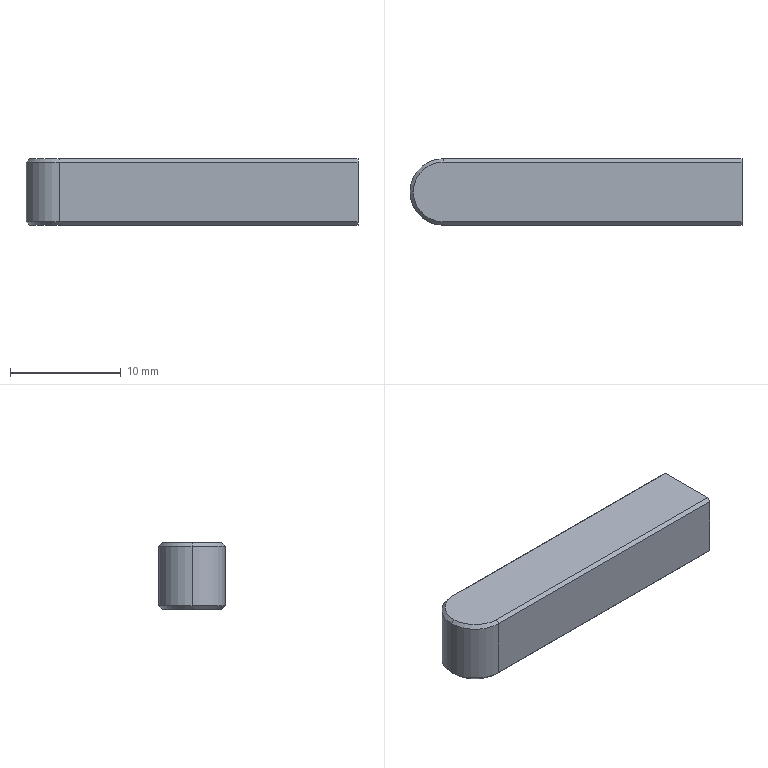Part | SolidWorks | features Chamfer 1, Extrusion 1, Fillet 1 | 1 solid | 15 faces | box 30 x 6 x 6 mm | volume 1051 mm3 | plane 9 | cone 4 | cylinder 2 | commonest cylinder face diameters 6 x2
STEP:
#1=CARTESIAN_POINT('',(15.,-2.7,0.));
#2=VERTEX_POINT('',#1);
#3=CARTESIAN_POINT('',(15.,2.7,0.));
#4=VERTEX_POINT('',#3);
#5=CARTESIAN_POINT('',(15.,3.,0.));
#6=DIRECTION('',(0.,1.,0.));
#7=VECTOR('',#6,1000.);
#8=LINE('',#5,#7);
#9=EDGE_CURVE('',#2,#4,#8,.T.);
#10=ORIENTED_EDGE('',*,*,#9,.T.);
#11=CARTESIAN_POINT('',(15.,3.,0.3));
#12=VERTEX_POINT('',#11);
#13=CARTESIAN_POINT('',(15.,3.,0.3));
#14=DIRECTION('',(0.,0.7071,0.7071));
#15=VECTOR('',#14,1000.);
#16=LINE('',#13,#15);
#17=EDGE_CURVE('',#4,#12,#16,.T.);
#18=ORIENTED_EDGE('',*,*,#17,.T.);
#19=CARTESIAN_POINT('',(15.,3.,5.7));
#20=VERTEX_POINT('',#19);
#21=CARTESIAN_POINT('',(15.,3.,6.));
#22=DIRECTION('',(0.,0.,-1.));
#23=VECTOR('',#22,1000.);
#24=LINE('',#21,#23);
#25=EDGE_CURVE('',#20,#12,#24,.T.);
#26=ORIENTED_EDGE('',*,*,#25,.F.);
#27=CARTESIAN_POINT('',(15.,2.7,6.));
#28=VERTEX_POINT('',#27);
#29=CARTESIAN_POINT('',(15.,2.7,6.));
#30=DIRECTION('',(0.,-0.7071,0.7071));
#31=VECTOR('',#30,1000.);
#32=LINE('',#29,#31);
#33=EDGE_CURVE('',#20,#28,#32,.T.);
#34=ORIENTED_EDGE('',*,*,#33,.T.);
#35=CARTESIAN_POINT('',(15.,-2.7,6.));
#36=VERTEX_POINT('',#35);
#37=CARTESIAN_POINT('',(15.,3.,6.));
#38=DIRECTION('',(0.,1.,0.));
#39=VECTOR('',#38,1000.);
#40=LINE('',#37,#39);
#41=EDGE_CURVE('',#36,#28,#40,.T.);
#42=ORIENTED_EDGE('',*,*,#41,.F.);
#43=CARTESIAN_POINT('',(15.,-3.,5.7));
#44=VERTEX_POINT('',#43);
#45=CARTESIAN_POINT('',(15.,-2.7,6.));
#46=DIRECTION('',(0.,-0.7071,-0.7071));
#47=VECTOR('',#46,1000.);
#48=LINE('',#45,#47);
#49=EDGE_CURVE('',#36,#44,#48,.T.);
#50=ORIENTED_EDGE('',*,*,#49,.T.);
#51=CARTESIAN_POINT('',(15.,-3.,0.3));
#52=VERTEX_POINT('',#51);
#53=CARTESIAN_POINT('',(15.,-3.,6.));
#54=DIRECTION('',(0.,0.,-1.));
#55=VECTOR('',#54,1000.);
#56=LINE('',#53,#55);
#57=EDGE_CURVE('',#44,#52,#56,.T.);
#58=ORIENTED_EDGE('',*,*,#57,.T.);
#59=CARTESIAN_POINT('',(15.,-3.,0.3));
#60=DIRECTION('',(0.,0.7071,-0.7071));
#61=VECTOR('',#60,1000.);
#62=LINE('',#59,#61);
#63=EDGE_CURVE('',#52,#2,#62,.T.);
#64=ORIENTED_EDGE('',*,*,#63,.T.);
#65=EDGE_LOOP('',(#10,#18,#26,#34,#42,#50,#58,#64));
#66=FACE_OUTER_BOUND('',#65,.T.);
#67=CARTESIAN_POINT('',(15.,3.,6.));
#68=DIRECTION('',(-1.,0.,0.));
#69=DIRECTION('',(0.,0.,1.));
#70=AXIS2_PLACEMENT_3D('',#67,#68,#69);
#71=PLANE('',#70);
#72=ADVANCED_FACE('',(#66),#71,.F.);
#73=ORIENTED_EDGE('',*,*,#25,.T.);
#74=CARTESIAN_POINT('',(-12.,3.,0.3));
#75=VERTEX_POINT('',#74);
#76=CARTESIAN_POINT('',(-15.,3.,0.3));
#77=DIRECTION('',(-1.,0.,0.));
#78=VECTOR('',#77,1000.);
#79=LINE('',#76,#78);
#80=EDGE_CURVE('',#12,#75,#79,.T.);
#81=ORIENTED_EDGE('',*,*,#80,.T.);
#82=CARTESIAN_POINT('',(-12.,3.,5.7));
#83=VERTEX_POINT('',#82);
#84=CARTESIAN_POINT('',(-12.,3.,6.));
#85=DIRECTION('',(0.,0.,1.));
#86=VECTOR('',#85,1000.);
#87=LINE('',#84,#86);
#88=EDGE_CURVE('',#75,#83,#87,.T.);
#89=ORIENTED_EDGE('',*,*,#88,.T.);
#90=CARTESIAN_POINT('',(15.,3.,5.7));
#91=DIRECTION('',(1.,0.,0.));
#92=VECTOR('',#91,1000.);
#93=LINE('',#90,#92);
#94=EDGE_CURVE('',#83,#20,#93,.T.);
#95=ORIENTED_EDGE('',*,*,#94,.T.);
#96=EDGE_LOOP('',(#73,#81,#89,#95));
#97=FACE_OUTER_BOUND('',#96,.T.);
#98=CARTESIAN_POINT('',(-15.,3.,6.));
#99=DIRECTION('',(0.,-1.,0.));
#100=DIRECTION('',(0.,0.,-1.));
#101=AXIS2_PLACEMENT_3D('',#98,#99,#100);
#102=PLANE('',#101);
#103=ADVANCED_FACE('',(#97),#102,.F.);
#104=CARTESIAN_POINT('',(-12.,-3.,5.7));
#105=VERTEX_POINT('',#104);
#106=CARTESIAN_POINT('',(-12.,-3.,0.3));
#107=VERTEX_POINT('',#106);
#108=CARTESIAN_POINT('',(-12.,-3.,6.));
#109=DIRECTION('',(0.,0.,-1.));
#110=VECTOR('',#109,1000.);
#111=LINE('',#108,#110);
#112=EDGE_CURVE('',#105,#107,#111,.T.);
#113=ORIENTED_EDGE('',*,*,#112,.T.);
#114=CARTESIAN_POINT('',(-15.,-3.,0.3));
#115=DIRECTION('',(1.,0.,0.));
#116=VECTOR('',#115,1000.);
#117=LINE('',#114,#116);
#118=EDGE_CURVE('',#107,#52,#117,.T.);
#119=ORIENTED_EDGE('',*,*,#118,.T.);
#120=ORIENTED_EDGE('',*,*,#57,.F.);
#121=CARTESIAN_POINT('',(-12.,-3.,5.7));
#122=DIRECTION('',(-1.,0.,0.));
#123=VECTOR('',#122,1000.);
#124=LINE('',#121,#123);
#125=EDGE_CURVE('',#44,#105,#124,.T.);
#126=ORIENTED_EDGE('',*,*,#125,.T.);
#127=EDGE_LOOP('',(#113,#119,#120,#126));
#128=FACE_OUTER_BOUND('',#127,.T.);
#129=CARTESIAN_POINT('',(-15.,-3.,6.));
#130=DIRECTION('',(0.,1.,0.));
#131=DIRECTION('',(0.,0.,1.));
#132=AXIS2_PLACEMENT_3D('',#129,#130,#131);
#133=PLANE('',#132);
#134=ADVANCED_FACE('',(#128),#133,.F.);
#135=ORIENTED_EDGE('',*,*,#41,.T.);
#136=CARTESIAN_POINT('',(-12.,2.7,6.));
#137=VERTEX_POINT('',#136);
#138=CARTESIAN_POINT('',(-12.,2.7,6.));
#139=DIRECTION('',(-1.,0.,0.));
#140=VECTOR('',#139,1000.);
#141=LINE('',#138,#140);
#142=EDGE_CURVE('',#28,#137,#141,.T.);
#143=ORIENTED_EDGE('',*,*,#142,.T.);
#144=CARTESIAN_POINT('',(-14.7,0.,6.));
#145=VERTEX_POINT('',#144);
#146=CARTESIAN_POINT('',(-12.,0.,6.));
#147=DIRECTION('',(0.,0.,1.));
#148=DIRECTION('',(1.,0.,0.));
#149=AXIS2_PLACEMENT_3D('',#146,#147,#148);
#150=CIRCLE('',#149,2.7);
#151=EDGE_CURVE('',#137,#145,#150,.T.);
#152=ORIENTED_EDGE('',*,*,#151,.T.);
#153=CARTESIAN_POINT('',(-12.,-2.7,6.));
#154=VERTEX_POINT('',#153);
#155=CARTESIAN_POINT('',(-12.,0.,6.));
#156=DIRECTION('',(0.,0.,1.));
#157=DIRECTION('',(1.,0.,0.));
#158=AXIS2_PLACEMENT_3D('',#155,#156,#157);
#159=CIRCLE('',#158,2.7);
#160=EDGE_CURVE('',#145,#154,#159,.T.);
#161=ORIENTED_EDGE('',*,*,#160,.T.);
#162=CARTESIAN_POINT('',(15.,-2.7,6.));
#163=DIRECTION('',(1.,0.,0.));
#164=VECTOR('',#163,1000.);
#165=LINE('',#162,#164);
#166=EDGE_CURVE('',#154,#36,#165,.T.);
#167=ORIENTED_EDGE('',*,*,#166,.T.);
#168=EDGE_LOOP('',(#135,#143,#152,#161,#167));
#169=FACE_OUTER_BOUND('',#168,.T.);
#170=CARTESIAN_POINT('',(0.,0.,6.));
#171=DIRECTION('',(0.,0.,1.));
#172=DIRECTION('',(1.,0.,0.));
#173=AXIS2_PLACEMENT_3D('',#170,#171,#172);
#174=PLANE('',#173);
#175=ADVANCED_FACE('',(#169),#174,.T.);
#176=CARTESIAN_POINT('',(-14.7,0.,0.));
#177=VERTEX_POINT('',#176);
#178=CARTESIAN_POINT('',(-12.,2.7,0.));
#179=VERTEX_POINT('',#178);
#180=CARTESIAN_POINT('',(-12.,0.,0.));
#181=DIRECTION('',(0.,0.,-1.));
#182=DIRECTION('',(1.,0.,0.));
#183=AXIS2_PLACEMENT_3D('',#180,#181,#182);
#184=CIRCLE('',#183,2.7);
#185=EDGE_CURVE('',#177,#179,#184,.T.);
#186=ORIENTED_EDGE('',*,*,#185,.T.);
#187=CARTESIAN_POINT('',(0.,2.7,0.));
#188=DIRECTION('',(1.,0.,0.));
#189=VECTOR('',#188,1000.);
#190=LINE('',#187,#189);
#191=EDGE_CURVE('',#179,#4,#190,.T.);
#192=ORIENTED_EDGE('',*,*,#191,.T.);
#193=ORIENTED_EDGE('',*,*,#9,.F.);
#194=CARTESIAN_POINT('',(-12.,-2.7,0.));
#195=VERTEX_POINT('',#194);
#196=CARTESIAN_POINT('',(0.,-2.7,0.));
#197=DIRECTION('',(-1.,0.,0.));
#198=VECTOR('',#197,1000.);
#199=LINE('',#196,#198);
#200=EDGE_CURVE('',#2,#195,#199,.T.);
#201=ORIENTED_EDGE('',*,*,#200,.T.);
#202=CARTESIAN_POINT('',(-12.,0.,0.));
#203=DIRECTION('',(0.,0.,-1.));
#204=DIRECTION('',(1.,0.,0.));
#205=AXIS2_PLACEMENT_3D('',#202,#203,#204);
#206=CIRCLE('',#205,2.7);
#207=EDGE_CURVE('',#195,#177,#206,.T.);
#208=ORIENTED_EDGE('',*,*,#207,.T.);
#209=EDGE_LOOP('',(#186,#192,#193,#201,#208));
#210=FACE_OUTER_BOUND('',#209,.T.);
#211=CARTESIAN_POINT('',(0.,0.,0.));
#212=DIRECTION('',(0.,0.,1.));
#213=DIRECTION('',(1.,0.,0.));
#214=AXIS2_PLACEMENT_3D('',#211,#212,#213);
#215=PLANE('',#214);
#216=ADVANCED_FACE('',(#210),#215,.F.);
#217=CARTESIAN_POINT('',(-15.,0.,0.3));
#218=VERTEX_POINT('',#217);
#219=CARTESIAN_POINT('',(-15.,0.,5.7));
#220=VERTEX_POINT('',#219);
#221=CARTESIAN_POINT('',(-15.,0.,6.));
#222=DIRECTION('',(0.,0.,1.));
#223=VECTOR('',#222,1000.);
#224=LINE('',#221,#223);
#225=EDGE_CURVE('',#218,#220,#224,.T.);
#226=ORIENTED_EDGE('',*,*,#225,.F.);
#227=CARTESIAN_POINT('',(-12.,0.,0.3));
#228=DIRECTION('',(0.,0.,1.));
#229=DIRECTION('',(1.,0.,0.));
#230=AXIS2_PLACEMENT_3D('',#227,#228,#229);
#231=CIRCLE('',#230,3.);
#232=EDGE_CURVE('',#218,#107,#231,.T.);
#233=ORIENTED_EDGE('',*,*,#232,.T.);
#234=ORIENTED_EDGE('',*,*,#112,.F.);
#235=CARTESIAN_POINT('',(-12.,0.,5.7));
#236=DIRECTION('',(0.,0.,-1.));
#237=DIRECTION('',(1.,0.,0.));
#238=AXIS2_PLACEMENT_3D('',#235,#236,#237);
#239=CIRCLE('',#238,3.);
#240=EDGE_CURVE('',#105,#220,#239,.T.);
#241=ORIENTED_EDGE('',*,*,#240,.T.);
#242=EDGE_LOOP('',(#226,#233,#234,#241));
#243=FACE_OUTER_BOUND('',#242,.T.);
#244=CARTESIAN_POINT('',(-12.,0.,6.));
#245=DIRECTION('',(0.,0.,-1.));
#246=DIRECTION('',(-1.,0.,0.));
#247=AXIS2_PLACEMENT_3D('',#244,#245,#246);
#248=CYLINDRICAL_SURFACE('',#247,3.);
#249=ADVANCED_FACE('',(#243),#248,.T.);
#250=ORIENTED_EDGE('',*,*,#88,.F.);
#251=CARTESIAN_POINT('',(-12.,0.,0.3));
#252=DIRECTION('',(0.,0.,1.));
#253=DIRECTION('',(1.,0.,0.));
#254=AXIS2_PLACEMENT_3D('',#251,#252,#253);
#255=CIRCLE('',#254,3.);
#256=EDGE_CURVE('',#75,#218,#255,.T.);
#257=ORIENTED_EDGE('',*,*,#256,.T.);
#258=ORIENTED_EDGE('',*,*,#225,.T.);
#259=CARTESIAN_POINT('',(-12.,0.,5.7));
#260=DIRECTION('',(0.,0.,-1.));
#261=DIRECTION('',(1.,0.,0.));
#262=AXIS2_PLACEMENT_3D('',#259,#260,#261);
#263=CIRCLE('',#262,3.);
#264=EDGE_CURVE('',#220,#83,#263,.T.);
#265=ORIENTED_EDGE('',*,*,#264,.T.);
#266=EDGE_LOOP('',(#250,#257,#258,#265));
#267=FACE_OUTER_BOUND('',#266,.T.);
#268=CARTESIAN_POINT('',(-12.,0.,6.));
#269=DIRECTION('',(0.,0.,-1.));
#270=DIRECTION('',(-1.,0.,0.));
#271=AXIS2_PLACEMENT_3D('',#268,#269,#270);
#272=CYLINDRICAL_SURFACE('',#271,3.);
#273=ADVANCED_FACE('',(#267),#272,.T.);
#274=ORIENTED_EDGE('',*,*,#63,.F.);
#275=ORIENTED_EDGE('',*,*,#118,.F.);
#276=CARTESIAN_POINT('',(-12.,-2.7,0.));
#277=DIRECTION('',(0.,-0.7071,0.7071));
#278=VECTOR('',#277,1000.);
#279=LINE('',#276,#278);
#280=EDGE_CURVE('',#195,#107,#279,.T.);
#281=ORIENTED_EDGE('',*,*,#280,.F.);
#282=ORIENTED_EDGE('',*,*,#200,.F.);
#283=EDGE_LOOP('',(#274,#275,#281,#282));
#284=FACE_OUTER_BOUND('',#283,.T.);
#285=CARTESIAN_POINT('',(-15.,-3.,0.3));
#286=DIRECTION('',(0.,0.7071,0.7071));
#287=DIRECTION('',(1.,0.,0.));
#288=AXIS2_PLACEMENT_3D('',#285,#286,#287);
#289=PLANE('',#288);
#290=ADVANCED_FACE('',(#284),#289,.F.);
#291=ORIENTED_EDGE('',*,*,#280,.T.);
#292=ORIENTED_EDGE('',*,*,#232,.F.);
#293=CARTESIAN_POINT('',(-14.7,0.,0.));
#294=DIRECTION('',(-0.7071,0.,0.7071));
#295=VECTOR('',#294,1000.);
#296=LINE('',#293,#295);
#297=EDGE_CURVE('',#177,#218,#296,.T.);
#298=ORIENTED_EDGE('',*,*,#297,.F.);
#299=ORIENTED_EDGE('',*,*,#207,.F.);
#300=EDGE_LOOP('',(#291,#292,#298,#299));
#301=FACE_OUTER_BOUND('',#300,.T.);
#302=CARTESIAN_POINT('',(-12.,0.,0.));
#303=DIRECTION('',(0.,0.,1.));
#304=DIRECTION('',(1.,0.,0.));
#305=AXIS2_PLACEMENT_3D('',#302,#303,#304);
#306=CONICAL_SURFACE('',#305,2.7,0.7854);
#307=ADVANCED_FACE('',(#301),#306,.T.);
#308=ORIENTED_EDGE('',*,*,#297,.T.);
#309=ORIENTED_EDGE('',*,*,#256,.F.);
#310=CARTESIAN_POINT('',(-12.,2.7,0.));
#311=DIRECTION('',(0.,0.7071,0.7071));
#312=VECTOR('',#311,1000.);
#313=LINE('',#310,#312);
#314=EDGE_CURVE('',#179,#75,#313,.T.);
#315=ORIENTED_EDGE('',*,*,#314,.F.);
#316=ORIENTED_EDGE('',*,*,#185,.F.);
#317=EDGE_LOOP('',(#308,#309,#315,#316));
#318=FACE_OUTER_BOUND('',#317,.T.);
#319=CARTESIAN_POINT('',(-12.,0.,0.));
#320=DIRECTION('',(0.,0.,1.));
#321=DIRECTION('',(1.,0.,0.));
#322=AXIS2_PLACEMENT_3D('',#319,#320,#321);
#323=CONICAL_SURFACE('',#322,2.7,0.7854);
#324=ADVANCED_FACE('',(#318),#323,.T.);
#325=ORIENTED_EDGE('',*,*,#17,.F.);
#326=ORIENTED_EDGE('',*,*,#191,.F.);
#327=ORIENTED_EDGE('',*,*,#314,.T.);
#328=ORIENTED_EDGE('',*,*,#80,.F.);
#329=EDGE_LOOP('',(#325,#326,#327,#328));
#330=FACE_OUTER_BOUND('',#329,.T.);
#331=CARTESIAN_POINT('',(-15.,3.,0.3));
#332=DIRECTION('',(0.,-0.7071,0.7071));
#333=DIRECTION('',(-1.,0.,0.));
#334=AXIS2_PLACEMENT_3D('',#331,#332,#333);
#335=PLANE('',#334);
#336=ADVANCED_FACE('',(#330),#335,.F.);
#337=ORIENTED_EDGE('',*,*,#49,.F.);
#338=ORIENTED_EDGE('',*,*,#166,.F.);
#339=CARTESIAN_POINT('',(-12.,-3.,5.7));
#340=DIRECTION('',(0.,0.7071,0.7071));
#341=VECTOR('',#340,1000.);
#342=LINE('',#339,#341);
#343=EDGE_CURVE('',#105,#154,#342,.T.);
#344=ORIENTED_EDGE('',*,*,#343,.F.);
#345=ORIENTED_EDGE('',*,*,#125,.F.);
#346=EDGE_LOOP('',(#337,#338,#344,#345));
#347=FACE_OUTER_BOUND('',#346,.T.);
#348=CARTESIAN_POINT('',(0.,-2.7,6.));
#349=DIRECTION('',(0.,-0.7071,0.7071));
#350=DIRECTION('',(-1.,0.,0.));
#351=AXIS2_PLACEMENT_3D('',#348,#349,#350);
#352=PLANE('',#351);
#353=ADVANCED_FACE('',(#347),#352,.T.);
#354=ORIENTED_EDGE('',*,*,#343,.T.);
#355=ORIENTED_EDGE('',*,*,#160,.F.);
#356=CARTESIAN_POINT('',(-15.,0.,5.7));
#357=DIRECTION('',(0.7071,0.,0.7071));
#358=VECTOR('',#357,1000.);
#359=LINE('',#356,#358);
#360=EDGE_CURVE('',#220,#145,#359,.T.);
#361=ORIENTED_EDGE('',*,*,#360,.F.);
#362=ORIENTED_EDGE('',*,*,#240,.F.);
#363=EDGE_LOOP('',(#354,#355,#361,#362));
#364=FACE_OUTER_BOUND('',#363,.T.);
#365=CARTESIAN_POINT('',(-12.,0.,6.));
#366=DIRECTION('',(0.,0.,-1.));
#367=DIRECTION('',(-1.,0.,0.));
#368=AXIS2_PLACEMENT_3D('',#365,#366,#367);
#369=CONICAL_SURFACE('',#368,2.7,0.7854);
#370=ADVANCED_FACE('',(#364),#369,.T.);
#371=ORIENTED_EDGE('',*,*,#360,.T.);
#372=ORIENTED_EDGE('',*,*,#151,.F.);
#373=CARTESIAN_POINT('',(-12.,3.,5.7));
#374=DIRECTION('',(0.,-0.7071,0.7071));
#375=VECTOR('',#374,1000.);
#376=LINE('',#373,#375);
#377=EDGE_CURVE('',#83,#137,#376,.T.);
#378=ORIENTED_EDGE('',*,*,#377,.F.);
#379=ORIENTED_EDGE('',*,*,#264,.F.);
#380=EDGE_LOOP('',(#371,#372,#378,#379));
#381=FACE_OUTER_BOUND('',#380,.T.);
#382=CARTESIAN_POINT('',(-12.,0.,6.));
#383=DIRECTION('',(0.,0.,-1.));
#384=DIRECTION('',(-1.,0.,0.));
#385=AXIS2_PLACEMENT_3D('',#382,#383,#384);
#386=CONICAL_SURFACE('',#385,2.7,0.7854);
#387=ADVANCED_FACE('',(#381),#386,.T.);
#388=ORIENTED_EDGE('',*,*,#33,.F.);
#389=ORIENTED_EDGE('',*,*,#94,.F.);
#390=ORIENTED_EDGE('',*,*,#377,.T.);
#391=ORIENTED_EDGE('',*,*,#142,.F.);
#392=EDGE_LOOP('',(#388,#389,#390,#391));
#393=FACE_OUTER_BOUND('',#392,.T.);
#394=CARTESIAN_POINT('',(0.,2.7,6.));
#395=DIRECTION('',(0.,0.7071,0.7071));
#396=DIRECTION('',(1.,0.,0.));
#397=AXIS2_PLACEMENT_3D('',#394,#395,#396);
#398=PLANE('',#397);
#399=ADVANCED_FACE('',(#393),#398,.T.);
#400=CLOSED_SHELL('',(#72,#103,#134,#175,#216,#249,#273,#290,#307,#324,#336,#353,#370,#387,#399));
#401=MANIFOLD_SOLID_BREP('',#400);
#402=CARTESIAN_POINT('',(0.,0.,0.));
#403=DIRECTION('',(0.,0.,1.));
#404=DIRECTION('',(1.,0.,0.));
#405=AXIS2_PLACEMENT_3D('',#402,#403,#404);
#406=(LENGTH_UNIT()NAMED_UNIT(*)SI_UNIT(.MILLI.,.METRE.));
#407=UNCERTAINTY_MEASURE_WITH_UNIT(LENGTH_MEASURE(0.00001),#406,'','');
#408=(NAMED_UNIT(*)PLANE_ANGLE_UNIT()SI_UNIT($,.RADIAN.));
#409=(NAMED_UNIT(*)SI_UNIT($,.STERADIAN.)SOLID_ANGLE_UNIT());
#410=(GEOMETRIC_REPRESENTATION_CONTEXT(3)GLOBAL_UNCERTAINTY_ASSIGNED_CONTEXT((#407))GLOBAL_UNIT_ASSIGNED_CONTEXT((#406,#408,#409))REPRESENTATION_CONTEXT('',''));
#411=ADVANCED_BREP_SHAPE_REPRESENTATION('',(#401,#405),#410);